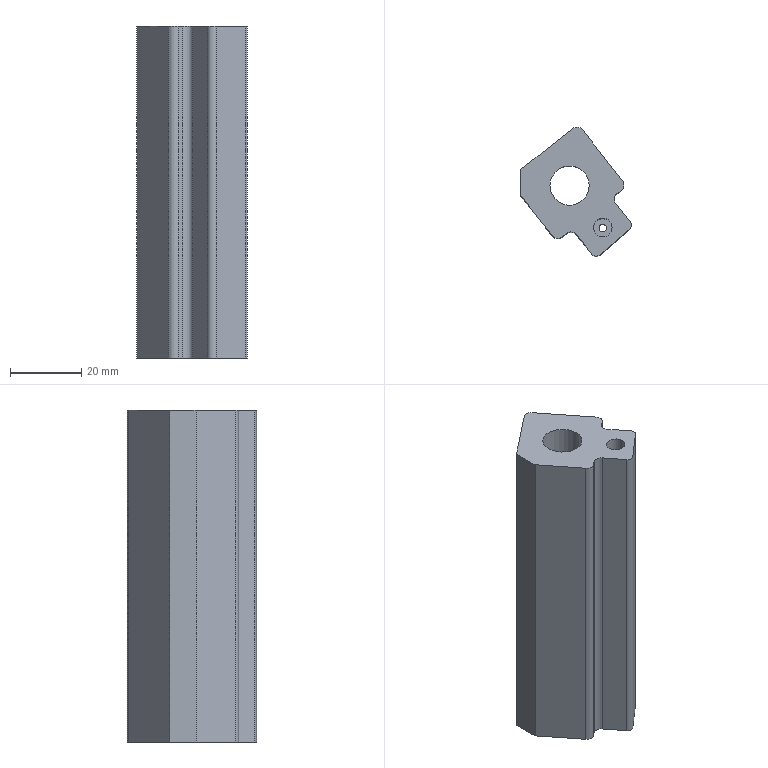Part | STEP file | gslz 2016.10.28-10_id2894_x_t | 1 solid | 24 faces | box 30.933 x 36.163 x 93 mm | volume 43152 mm3 | plane 12 | cylinder 11 | spline 1 | commonest cylinder face diameters 4 x5 3 x2 2.1 x1 5.2 x1 11 x1 17 x1